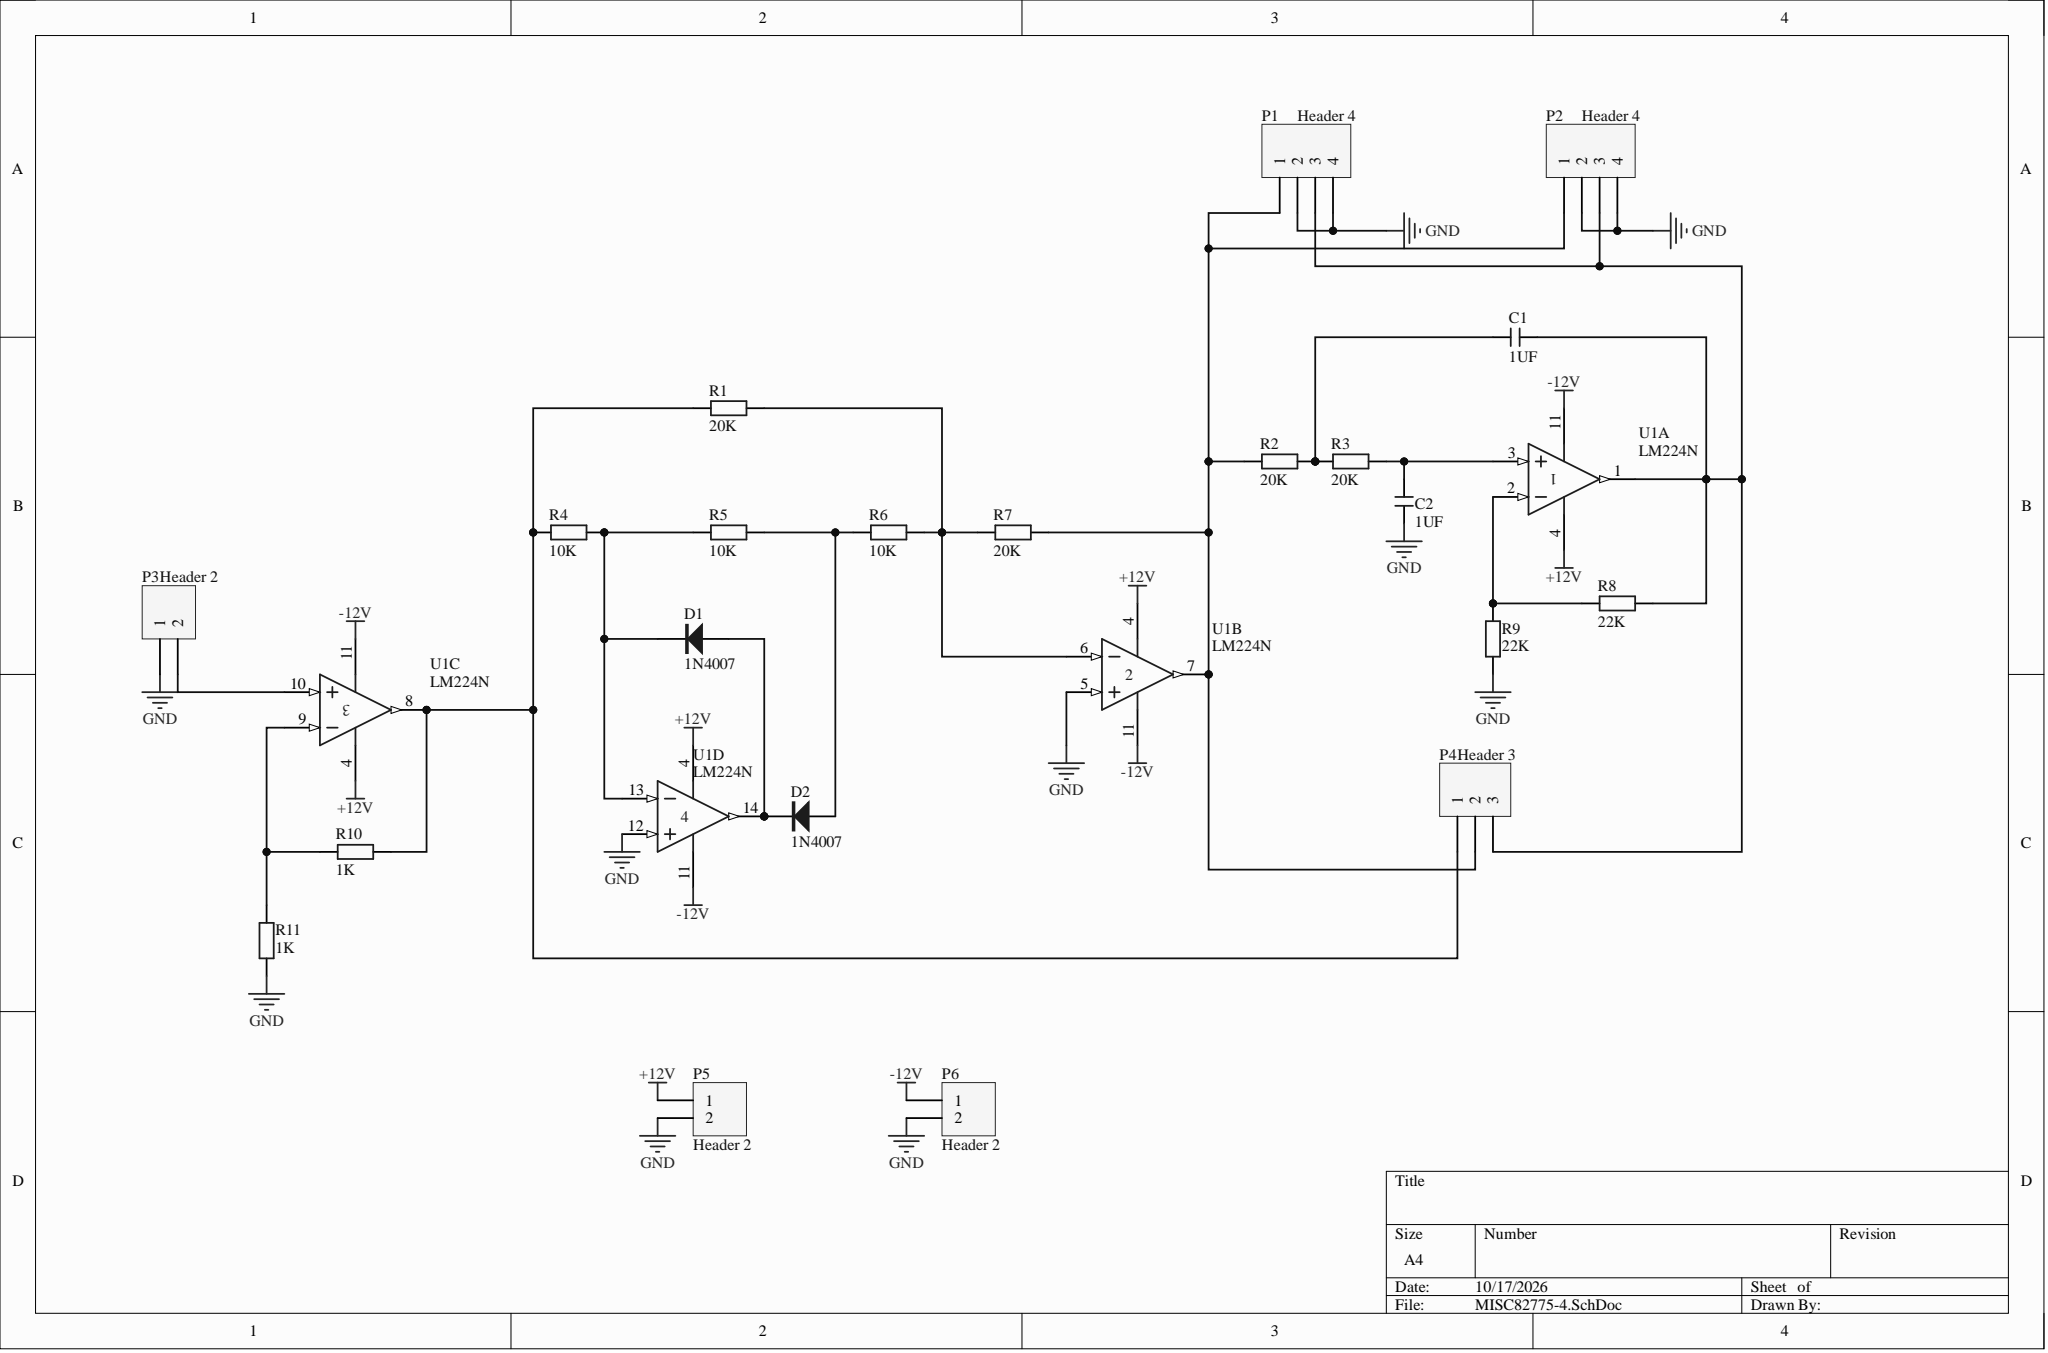Circuit board | Altium Designer | 22 parts | 15 nets
Bill of materials:
Comment,Description,Designator,Footprint,LibRef,Quantity
"1UF","Ceramic capacitor","C1, C2","CC 1.8*3.6","CC","2"
"1N4007","Rectifier diode","D1, D2","DO-41","1N4007","2"
"Header 4","Header, 4-Pin","P1, P2","HDR1X4","Header 4","2"
"Header 2","Header, 2-Pin","P3, P5, P6","HDR1X2","Header 2","3"
"Header 3","Header, 3-Pin","P4","HDR1X3","Header 3","1"
"20K","Color-band resistor","R1, R2, R3, R7","RS 1/4W","R-S","4"
"10K","Color-band resistor","R4, R5, R6","RS 1/4W","R-S","3"
"22K","Color-band resistor","R8, R9","RS 1/4W","R-S","2"
"1K","Color-band resistor","R10, R11","RS 1/4W","R-S","2"
"LM224N","Quad Low-Power Operational Amplifier","U1","646-06","LM224N","1"
Netlist (Protel format):
[
C1
CC 1.8*3.6
1UF



]
[
C2
CC 1.8*3.6
1UF



]
[
D1
DO-41
1N4007



]
[
D2
DO-41
1N4007



]
[
P1
HDR1X4
Header 4



]
[
P2
HDR1X4
Header 4



]
[
P3
HDR1X2
Header 2



]
[
P4
HDR1X3
Header 3



]
[
P5
HDR1X2
Header 2



]
[
P6
HDR1X2
Header 2



]
[
R1
RS 1/4W
20K



]
[
R2
RS 1/4W
20K



]
[
R3
RS 1/4W
20K



]
[
R4
RS 1/4W
10K



]
[
R5
RS 1/4W
10K



]
[
R6
RS 1/4W
10K



]
[
R7
RS 1/4W
20K



]
[
R8
RS 1/4W
22K



]
[
R9
RS 1/4W
22K



]
[
R10
RS 1/4W
1K



]
[
R11
RS 1/4W
1K



]
[
U1
646-06
LM224N



]
(
NetR10_1
R10-1
R11-2
U1-9
)
(
NetR8_1
R8-1
R9-2
U1-2
)
(
NetR1_2
R1-2
R6-2
R7-1
U1-6
)
(
NetP4_1
P4-1
R1-1
R4-1
R10-2
U1-8
)
(
NetP3_2
P3-2
U1-10
)
(
NetP1_1
P1-1
P2-1
P4-2
R2-1
R7-2
U1-7
)
(
NetD2_1
D2-1
R5-2
R6-1
)
(
NetD1_2
D1-2
R4-2
R5-1
U1-13
)
(
NetD1_1
D1-1
D2-2
U1-14
)
(
NetC2_1
C2-1
R3-2
U1-3
)
(
NetC1_2
C1-2
P1-3
P2-3
P4-3
R8-2
U1-1
)
(
NetC1_1
C1-1
R2-2
R3-1
)
(
GND
C2-2
P1-2
P1-4
P2-2
P2-4
P3-1
P5-2
P6-2
R9-1
R11-1
U1-5
U1-12
)
(
-12V
P6-1
U1-11
)
(
+12V
P5-1
U1-4
)